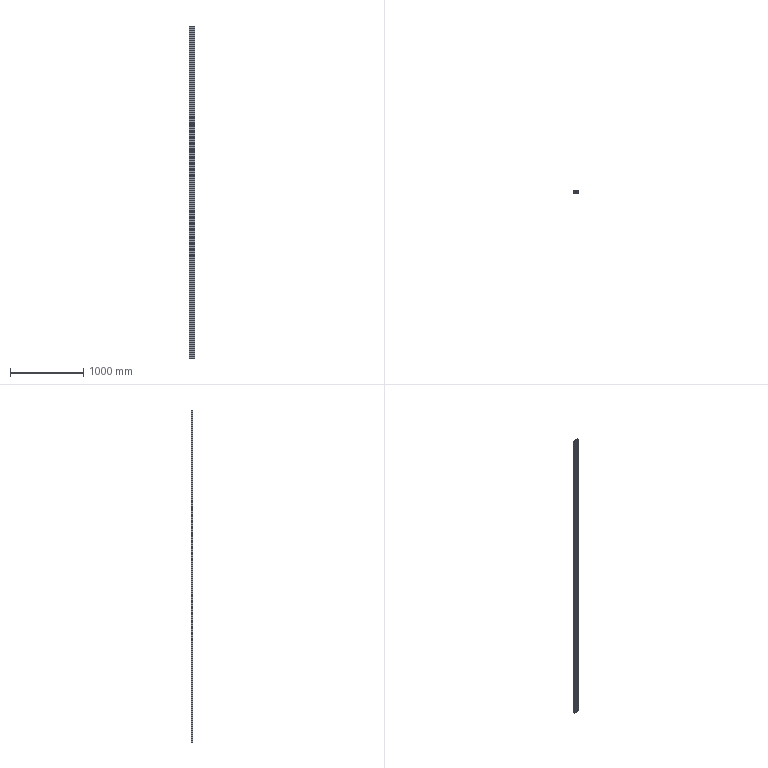Part | SolidWorks | features MBimport 1, MoveFace 1 | 1 solid | 286 faces | box 80 x 20 x 4546 mm | volume 2507089 mm3 | plane 182 | cylinder 104 | commonest cylinder face diameters 0.6 x40 3 x36 0.4 x20 5 x8